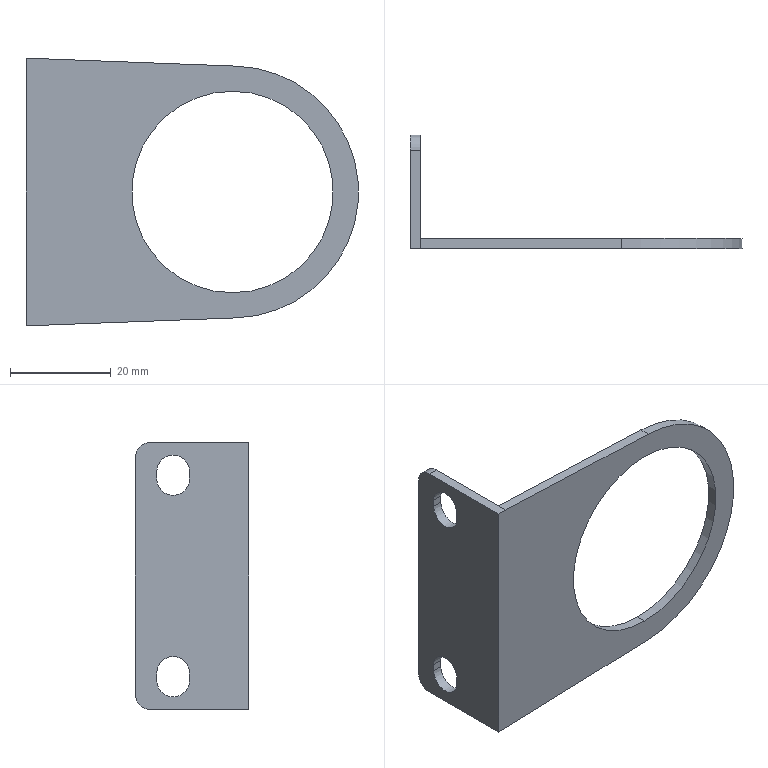Part | SolidWorks | features BaseBody 1 | 1 solid | 24 faces | box 66 x 22.5 x 53 mm | volume 5674 mm3 | plane 13 | cylinder 11 | commonest cylinder face diameters 6.5 x6 6 x2 40 x2 50 x1
STEP:
#1=CARTESIAN_POINT('',(0.,33.,20.));
#2=VERTEX_POINT('',#1);
#3=CARTESIAN_POINT('',(0.,33.,-20.));
#4=VERTEX_POINT('',#3);
#5=CARTESIAN_POINT('',(0.,33.,0.));
#6=DIRECTION('',(0.,-1.,0.));
#7=DIRECTION('',(0.,0.,-1.));
#8=AXIS2_PLACEMENT_3D('',#5,#6,#7);
#9=CIRCLE('',#8,20.);
#10=EDGE_CURVE('',#2,#4,#9,.T.);
#11=ORIENTED_EDGE('',*,*,#10,.F.);
#12=CARTESIAN_POINT('',(0.,31.,20.));
#13=VERTEX_POINT('',#12);
#14=CARTESIAN_POINT('',(0.,31.,20.));
#15=DIRECTION('',(0.,-1.,0.));
#16=VECTOR('',#15,1000.);
#17=LINE('',#14,#16);
#18=EDGE_CURVE('',#2,#13,#17,.T.);
#19=ORIENTED_EDGE('',*,*,#18,.T.);
#20=CARTESIAN_POINT('',(0.,31.,-20.));
#21=VERTEX_POINT('',#20);
#22=CARTESIAN_POINT('',(0.,31.,0.));
#23=DIRECTION('',(0.,1.,0.));
#24=DIRECTION('',(0.,0.,-1.));
#25=AXIS2_PLACEMENT_3D('',#22,#23,#24);
#26=CIRCLE('',#25,20.);
#27=EDGE_CURVE('',#21,#13,#26,.T.);
#28=ORIENTED_EDGE('',*,*,#27,.F.);
#29=CARTESIAN_POINT('',(0.,31.,-20.));
#30=DIRECTION('',(0.,-1.,0.));
#31=VECTOR('',#30,1000.);
#32=LINE('',#29,#31);
#33=EDGE_CURVE('',#4,#21,#32,.T.);
#34=ORIENTED_EDGE('',*,*,#33,.F.);
#35=EDGE_LOOP('',(#11,#19,#28,#34));
#36=FACE_OUTER_BOUND('',#35,.T.);
#37=CARTESIAN_POINT('',(0.,31.,0.));
#38=DIRECTION('',(0.,-1.,0.));
#39=DIRECTION('',(0.,0.,-1.));
#40=AXIS2_PLACEMENT_3D('',#37,#38,#39);
#41=CYLINDRICAL_SURFACE('',#40,20.);
#42=ADVANCED_FACE('',(#36),#41,.F.);
#43=CARTESIAN_POINT('',(-39.,46.,24.));
#44=VERTEX_POINT('',#43);
#45=CARTESIAN_POINT('',(-39.,49.25,20.75));
#46=VERTEX_POINT('',#45);
#47=CARTESIAN_POINT('',(-39.,46.,20.75));
#48=DIRECTION('',(-1.,0.,0.));
#49=DIRECTION('',(0.,0.,1.));
#50=AXIS2_PLACEMENT_3D('',#47,#48,#49);
#51=CIRCLE('',#50,3.25);
#52=EDGE_CURVE('',#44,#46,#51,.T.);
#53=ORIENTED_EDGE('',*,*,#52,.F.);
#54=CARTESIAN_POINT('',(-41.,46.,24.));
#55=VERTEX_POINT('',#54);
#56=CARTESIAN_POINT('',(-41.,46.,24.));
#57=DIRECTION('',(-1.,0.,0.));
#58=VECTOR('',#57,1000.);
#59=LINE('',#56,#58);
#60=EDGE_CURVE('',#44,#55,#59,.T.);
#61=ORIENTED_EDGE('',*,*,#60,.T.);
#62=CARTESIAN_POINT('',(-41.,49.25,20.75));
#63=VERTEX_POINT('',#62);
#64=CARTESIAN_POINT('',(-41.,46.,20.75));
#65=DIRECTION('',(-1.,0.,0.));
#66=DIRECTION('',(0.,0.,1.));
#67=AXIS2_PLACEMENT_3D('',#64,#65,#66);
#68=CIRCLE('',#67,3.25);
#69=EDGE_CURVE('',#55,#63,#68,.T.);
#70=ORIENTED_EDGE('',*,*,#69,.T.);
#71=CARTESIAN_POINT('',(-41.,49.25,20.75));
#72=DIRECTION('',(-1.,0.,0.));
#73=VECTOR('',#72,1000.);
#74=LINE('',#71,#73);
#75=EDGE_CURVE('',#46,#63,#74,.T.);
#76=ORIENTED_EDGE('',*,*,#75,.F.);
#77=EDGE_LOOP('',(#53,#61,#70,#76));
#78=FACE_OUTER_BOUND('',#77,.T.);
#79=CARTESIAN_POINT('',(-41.,46.,20.75));
#80=DIRECTION('',(-1.,0.,0.));
#81=DIRECTION('',(0.,0.,1.));
#82=AXIS2_PLACEMENT_3D('',#79,#80,#81);
#83=CYLINDRICAL_SURFACE('',#82,3.25);
#84=ADVANCED_FACE('',(#78),#83,.F.);
#85=CARTESIAN_POINT('',(-39.,46.,-16.));
#86=VERTEX_POINT('',#85);
#87=CARTESIAN_POINT('',(-39.,49.25,-19.25));
#88=VERTEX_POINT('',#87);
#89=CARTESIAN_POINT('',(-39.,46.,-19.25));
#90=DIRECTION('',(-1.,0.,0.));
#91=DIRECTION('',(0.,0.,1.));
#92=AXIS2_PLACEMENT_3D('',#89,#90,#91);
#93=CIRCLE('',#92,3.25);
#94=EDGE_CURVE('',#86,#88,#93,.T.);
#95=ORIENTED_EDGE('',*,*,#94,.F.);
#96=CARTESIAN_POINT('',(-41.,46.,-16.));
#97=VERTEX_POINT('',#96);
#98=CARTESIAN_POINT('',(-41.,46.,-16.));
#99=DIRECTION('',(-1.,0.,0.));
#100=VECTOR('',#99,1000.);
#101=LINE('',#98,#100);
#102=EDGE_CURVE('',#86,#97,#101,.T.);
#103=ORIENTED_EDGE('',*,*,#102,.T.);
#104=CARTESIAN_POINT('',(-41.,49.25,-19.25));
#105=VERTEX_POINT('',#104);
#106=CARTESIAN_POINT('',(-41.,46.,-19.25));
#107=DIRECTION('',(-1.,0.,0.));
#108=DIRECTION('',(0.,0.,1.));
#109=AXIS2_PLACEMENT_3D('',#106,#107,#108);
#110=CIRCLE('',#109,3.25);
#111=EDGE_CURVE('',#97,#105,#110,.T.);
#112=ORIENTED_EDGE('',*,*,#111,.T.);
#113=CARTESIAN_POINT('',(-41.,49.25,-19.25));
#114=DIRECTION('',(-1.,0.,0.));
#115=VECTOR('',#114,1000.);
#116=LINE('',#113,#115);
#117=EDGE_CURVE('',#88,#105,#116,.T.);
#118=ORIENTED_EDGE('',*,*,#117,.F.);
#119=EDGE_LOOP('',(#95,#103,#112,#118));
#120=FACE_OUTER_BOUND('',#119,.T.);
#121=CARTESIAN_POINT('',(-41.,46.,-19.25));
#122=DIRECTION('',(-1.,0.,0.));
#123=DIRECTION('',(0.,0.,1.));
#124=AXIS2_PLACEMENT_3D('',#121,#122,#123);
#125=CYLINDRICAL_SURFACE('',#124,3.25);
#126=ADVANCED_FACE('',(#120),#125,.F.);
#127=CARTESIAN_POINT('',(-41.,49.25,-20.75));
#128=VERTEX_POINT('',#127);
#129=CARTESIAN_POINT('',(-41.,49.25,-20.75));
#130=DIRECTION('',(0.,0.,-1.));
#131=VECTOR('',#130,1000.);
#132=LINE('',#129,#131);
#133=EDGE_CURVE('',#105,#128,#132,.T.);
#134=ORIENTED_EDGE('',*,*,#133,.T.);
#135=CARTESIAN_POINT('',(-39.,49.25,-20.75));
#136=VERTEX_POINT('',#135);
#137=CARTESIAN_POINT('',(-41.,49.25,-20.75));
#138=DIRECTION('',(1.,0.,0.));
#139=VECTOR('',#138,1000.);
#140=LINE('',#137,#139);
#141=EDGE_CURVE('',#128,#136,#140,.T.);
#142=ORIENTED_EDGE('',*,*,#141,.T.);
#143=CARTESIAN_POINT('',(-39.,49.25,-20.75));
#144=DIRECTION('',(0.,0.,1.));
#145=VECTOR('',#144,1000.);
#146=LINE('',#143,#145);
#147=EDGE_CURVE('',#136,#88,#146,.T.);
#148=ORIENTED_EDGE('',*,*,#147,.T.);
#149=ORIENTED_EDGE('',*,*,#117,.T.);
#150=EDGE_LOOP('',(#134,#142,#148,#149));
#151=FACE_OUTER_BOUND('',#150,.T.);
#152=CARTESIAN_POINT('',(-41.,49.25,-20.75));
#153=DIRECTION('',(0.,-1.,0.));
#154=DIRECTION('',(0.,0.,-1.));
#155=AXIS2_PLACEMENT_3D('',#152,#153,#154);
#156=PLANE('',#155);
#157=ADVANCED_FACE('',(#151),#156,.T.);
#158=CARTESIAN_POINT('',(-41.,42.75,-20.75));
#159=VERTEX_POINT('',#158);
#160=CARTESIAN_POINT('',(-41.,42.75,-19.25));
#161=VERTEX_POINT('',#160);
#162=CARTESIAN_POINT('',(-41.,42.75,-19.25));
#163=DIRECTION('',(0.,0.,1.));
#164=VECTOR('',#163,1000.);
#165=LINE('',#162,#164);
#166=EDGE_CURVE('',#159,#161,#165,.T.);
#167=ORIENTED_EDGE('',*,*,#166,.T.);
#168=CARTESIAN_POINT('',(-39.,42.75,-19.25));
#169=VERTEX_POINT('',#168);
#170=CARTESIAN_POINT('',(-41.,42.75,-19.25));
#171=DIRECTION('',(1.,0.,0.));
#172=VECTOR('',#171,1000.);
#173=LINE('',#170,#172);
#174=EDGE_CURVE('',#161,#169,#173,.T.);
#175=ORIENTED_EDGE('',*,*,#174,.T.);
#176=CARTESIAN_POINT('',(-39.,42.75,-20.75));
#177=VERTEX_POINT('',#176);
#178=CARTESIAN_POINT('',(-39.,42.75,-19.25));
#179=DIRECTION('',(0.,0.,-1.));
#180=VECTOR('',#179,1000.);
#181=LINE('',#178,#180);
#182=EDGE_CURVE('',#169,#177,#181,.T.);
#183=ORIENTED_EDGE('',*,*,#182,.T.);
#184=CARTESIAN_POINT('',(-41.,42.75,-20.75));
#185=DIRECTION('',(-1.,0.,0.));
#186=VECTOR('',#185,1000.);
#187=LINE('',#184,#186);
#188=EDGE_CURVE('',#177,#159,#187,.T.);
#189=ORIENTED_EDGE('',*,*,#188,.T.);
#190=EDGE_LOOP('',(#167,#175,#183,#189));
#191=FACE_OUTER_BOUND('',#190,.T.);
#192=CARTESIAN_POINT('',(-41.,42.75,-19.25));
#193=DIRECTION('',(0.,1.,0.));
#194=DIRECTION('',(1.,0.,0.));
#195=AXIS2_PLACEMENT_3D('',#192,#193,#194);
#196=PLANE('',#195);
#197=ADVANCED_FACE('',(#191),#196,.T.);
#198=CARTESIAN_POINT('',(-41.,49.25,19.25));
#199=VERTEX_POINT('',#198);
#200=CARTESIAN_POINT('',(-41.,49.25,19.25));
#201=DIRECTION('',(0.,0.,-1.));
#202=VECTOR('',#201,1000.);
#203=LINE('',#200,#202);
#204=EDGE_CURVE('',#63,#199,#203,.T.);
#205=ORIENTED_EDGE('',*,*,#204,.T.);
#206=CARTESIAN_POINT('',(-39.,49.25,19.25));
#207=VERTEX_POINT('',#206);
#208=CARTESIAN_POINT('',(-41.,49.25,19.25));
#209=DIRECTION('',(1.,0.,0.));
#210=VECTOR('',#209,1000.);
#211=LINE('',#208,#210);
#212=EDGE_CURVE('',#199,#207,#211,.T.);
#213=ORIENTED_EDGE('',*,*,#212,.T.);
#214=CARTESIAN_POINT('',(-39.,49.25,19.25));
#215=DIRECTION('',(0.,0.,1.));
#216=VECTOR('',#215,1000.);
#217=LINE('',#214,#216);
#218=EDGE_CURVE('',#207,#46,#217,.T.);
#219=ORIENTED_EDGE('',*,*,#218,.T.);
#220=ORIENTED_EDGE('',*,*,#75,.T.);
#221=EDGE_LOOP('',(#205,#213,#219,#220));
#222=FACE_OUTER_BOUND('',#221,.T.);
#223=CARTESIAN_POINT('',(-41.,49.25,19.25));
#224=DIRECTION('',(0.,-1.,0.));
#225=DIRECTION('',(0.,0.,-1.));
#226=AXIS2_PLACEMENT_3D('',#223,#224,#225);
#227=PLANE('',#226);
#228=ADVANCED_FACE('',(#222),#227,.T.);
#229=CARTESIAN_POINT('',(-41.,42.75,19.25));
#230=VERTEX_POINT('',#229);
#231=CARTESIAN_POINT('',(-41.,42.75,20.75));
#232=VERTEX_POINT('',#231);
#233=CARTESIAN_POINT('',(-41.,42.75,20.75));
#234=DIRECTION('',(0.,0.,1.));
#235=VECTOR('',#234,1000.);
#236=LINE('',#233,#235);
#237=EDGE_CURVE('',#230,#232,#236,.T.);
#238=ORIENTED_EDGE('',*,*,#237,.T.);
#239=CARTESIAN_POINT('',(-39.,42.75,20.75));
#240=VERTEX_POINT('',#239);
#241=CARTESIAN_POINT('',(-41.,42.75,20.75));
#242=DIRECTION('',(1.,0.,0.));
#243=VECTOR('',#242,1000.);
#244=LINE('',#241,#243);
#245=EDGE_CURVE('',#232,#240,#244,.T.);
#246=ORIENTED_EDGE('',*,*,#245,.T.);
#247=CARTESIAN_POINT('',(-39.,42.75,19.25));
#248=VERTEX_POINT('',#247);
#249=CARTESIAN_POINT('',(-39.,42.75,20.75));
#250=DIRECTION('',(0.,0.,-1.));
#251=VECTOR('',#250,1000.);
#252=LINE('',#249,#251);
#253=EDGE_CURVE('',#240,#248,#252,.T.);
#254=ORIENTED_EDGE('',*,*,#253,.T.);
#255=CARTESIAN_POINT('',(-41.,42.75,19.25));
#256=DIRECTION('',(-1.,0.,0.));
#257=VECTOR('',#256,1000.);
#258=LINE('',#255,#257);
#259=EDGE_CURVE('',#248,#230,#258,.T.);
#260=ORIENTED_EDGE('',*,*,#259,.T.);
#261=EDGE_LOOP('',(#238,#246,#254,#260));
#262=FACE_OUTER_BOUND('',#261,.T.);
#263=CARTESIAN_POINT('',(-41.,42.75,20.75));
#264=DIRECTION('',(0.,1.,0.));
#265=DIRECTION('',(1.,0.,0.));
#266=AXIS2_PLACEMENT_3D('',#263,#264,#265);
#267=PLANE('',#266);
#268=ADVANCED_FACE('',(#262),#267,.T.);
#269=CARTESIAN_POINT('',(-41.,53.5,-23.5));
#270=VERTEX_POINT('',#269);
#271=CARTESIAN_POINT('',(-41.,53.5,23.5));
#272=VERTEX_POINT('',#271);
#273=CARTESIAN_POINT('',(-41.,53.5,0.));
#274=DIRECTION('',(0.,0.,1.));
#275=VECTOR('',#274,1000.);
#276=LINE('',#273,#275);
#277=EDGE_CURVE('',#270,#272,#276,.T.);
#278=ORIENTED_EDGE('',*,*,#277,.T.);
#279=CARTESIAN_POINT('',(-39.,53.5,23.5));
#280=VERTEX_POINT('',#279);
#281=CARTESIAN_POINT('',(-41.,53.5,23.5));
#282=DIRECTION('',(-1.,0.,0.));
#283=VECTOR('',#282,1000.);
#284=LINE('',#281,#283);
#285=EDGE_CURVE('',#280,#272,#284,.T.);
#286=ORIENTED_EDGE('',*,*,#285,.F.);
#287=CARTESIAN_POINT('',(-39.,53.5,-23.5));
#288=VERTEX_POINT('',#287);
#289=CARTESIAN_POINT('',(-39.,53.5,0.));
#290=DIRECTION('',(0.,0.,1.));
#291=VECTOR('',#290,1000.);
#292=LINE('',#289,#291);
#293=EDGE_CURVE('',#288,#280,#292,.T.);
#294=ORIENTED_EDGE('',*,*,#293,.F.);
#295=CARTESIAN_POINT('',(-41.,53.5,-23.5));
#296=DIRECTION('',(1.,0.,0.));
#297=VECTOR('',#296,1000.);
#298=LINE('',#295,#297);
#299=EDGE_CURVE('',#270,#288,#298,.T.);
#300=ORIENTED_EDGE('',*,*,#299,.F.);
#301=EDGE_LOOP('',(#278,#286,#294,#300));
#302=FACE_OUTER_BOUND('',#301,.T.);
#303=CARTESIAN_POINT('',(-41.,53.5,23.5));
#304=DIRECTION('',(0.,1.,0.));
#305=DIRECTION('',(1.,0.,0.));
#306=AXIS2_PLACEMENT_3D('',#303,#304,#305);
#307=PLANE('',#306);
#308=ADVANCED_FACE('',(#302),#307,.T.);
#309=CARTESIAN_POINT('',(-41.,50.5,26.5));
#310=VERTEX_POINT('',#309);
#311=CARTESIAN_POINT('',(-41.,50.5,23.5));
#312=DIRECTION('',(1.,0.,0.));
#313=DIRECTION('',(0.,0.,1.));
#314=AXIS2_PLACEMENT_3D('',#311,#312,#313);
#315=CIRCLE('',#314,3.);
#316=EDGE_CURVE('',#272,#310,#315,.T.);
#317=ORIENTED_EDGE('',*,*,#316,.T.);
#318=CARTESIAN_POINT('',(-39.,50.5,26.5));
#319=VERTEX_POINT('',#318);
#320=CARTESIAN_POINT('',(-41.,50.5,26.5));
#321=DIRECTION('',(-1.,0.,0.));
#322=VECTOR('',#321,1000.);
#323=LINE('',#320,#322);
#324=EDGE_CURVE('',#319,#310,#323,.T.);
#325=ORIENTED_EDGE('',*,*,#324,.F.);
#326=CARTESIAN_POINT('',(-39.,50.5,23.5));
#327=DIRECTION('',(1.,0.,0.));
#328=DIRECTION('',(0.,0.,1.));
#329=AXIS2_PLACEMENT_3D('',#326,#327,#328);
#330=CIRCLE('',#329,3.);
#331=EDGE_CURVE('',#280,#319,#330,.T.);
#332=ORIENTED_EDGE('',*,*,#331,.F.);
#333=ORIENTED_EDGE('',*,*,#285,.T.);
#334=EDGE_LOOP('',(#317,#325,#332,#333));
#335=FACE_OUTER_BOUND('',#334,.T.);
#336=CARTESIAN_POINT('',(-41.,50.5,23.5));
#337=DIRECTION('',(-1.,0.,0.));
#338=DIRECTION('',(0.,0.,1.));
#339=AXIS2_PLACEMENT_3D('',#336,#337,#338);
#340=CYLINDRICAL_SURFACE('',#339,3.);
#341=ADVANCED_FACE('',(#335),#340,.T.);
#342=ORIENTED_EDGE('',*,*,#141,.F.);
#343=CARTESIAN_POINT('',(-41.,46.,-20.75));
#344=DIRECTION('',(-1.,0.,0.));
#345=DIRECTION('',(0.,0.,1.));
#346=AXIS2_PLACEMENT_3D('',#343,#344,#345);
#347=CIRCLE('',#346,3.25);
#348=EDGE_CURVE('',#128,#159,#347,.T.);
#349=ORIENTED_EDGE('',*,*,#348,.T.);
#350=ORIENTED_EDGE('',*,*,#188,.F.);
#351=CARTESIAN_POINT('',(-39.,46.,-20.75));
#352=DIRECTION('',(-1.,0.,0.));
#353=DIRECTION('',(0.,0.,1.));
#354=AXIS2_PLACEMENT_3D('',#351,#352,#353);
#355=CIRCLE('',#354,3.25);
#356=EDGE_CURVE('',#136,#177,#355,.T.);
#357=ORIENTED_EDGE('',*,*,#356,.F.);
#358=EDGE_LOOP('',(#342,#349,#350,#357));
#359=FACE_OUTER_BOUND('',#358,.T.);
#360=CARTESIAN_POINT('',(-41.,46.,-20.75));
#361=DIRECTION('',(-1.,0.,0.));
#362=DIRECTION('',(0.,0.,1.));
#363=AXIS2_PLACEMENT_3D('',#360,#361,#362);
#364=CYLINDRICAL_SURFACE('',#363,3.25);
#365=ADVANCED_FACE('',(#359),#364,.F.);
#366=ORIENTED_EDGE('',*,*,#212,.F.);
#367=CARTESIAN_POINT('',(-41.,46.,19.25));
#368=DIRECTION('',(-1.,0.,0.));
#369=DIRECTION('',(0.,0.,1.));
#370=AXIS2_PLACEMENT_3D('',#367,#368,#369);
#371=CIRCLE('',#370,3.25);
#372=EDGE_CURVE('',#199,#230,#371,.T.);
#373=ORIENTED_EDGE('',*,*,#372,.T.);
#374=ORIENTED_EDGE('',*,*,#259,.F.);
#375=CARTESIAN_POINT('',(-39.,46.,19.25));
#376=DIRECTION('',(-1.,0.,0.));
#377=DIRECTION('',(0.,0.,1.));
#378=AXIS2_PLACEMENT_3D('',#375,#376,#377);
#379=CIRCLE('',#378,3.25);
#380=EDGE_CURVE('',#207,#248,#379,.T.);
#381=ORIENTED_EDGE('',*,*,#380,.F.);
#382=EDGE_LOOP('',(#366,#373,#374,#381));
#383=FACE_OUTER_BOUND('',#382,.T.);
#384=CARTESIAN_POINT('',(-41.,46.,19.25));
#385=DIRECTION('',(-1.,0.,0.));
#386=DIRECTION('',(0.,0.,1.));
#387=AXIS2_PLACEMENT_3D('',#384,#385,#386);
#388=CYLINDRICAL_SURFACE('',#387,3.25);
#389=ADVANCED_FACE('',(#383),#388,.F.);
#390=ORIENTED_EDGE('',*,*,#380,.T.);
#391=ORIENTED_EDGE('',*,*,#253,.F.);
#392=CARTESIAN_POINT('',(-39.,46.,20.75));
#393=DIRECTION('',(-1.,0.,0.));
#394=DIRECTION('',(0.,0.,1.));
#395=AXIS2_PLACEMENT_3D('',#392,#393,#394);
#396=CIRCLE('',#395,3.25);
#397=EDGE_CURVE('',#240,#44,#396,.T.);
#398=ORIENTED_EDGE('',*,*,#397,.T.);
#399=ORIENTED_EDGE('',*,*,#52,.T.);
#400=ORIENTED_EDGE('',*,*,#218,.F.);
#401=EDGE_LOOP('',(#390,#391,#398,#399,#400));
#402=FACE_BOUND('',#401,.T.);
#403=ORIENTED_EDGE('',*,*,#356,.T.);
#404=ORIENTED_EDGE('',*,*,#182,.F.);
#405=CARTESIAN_POINT('',(-39.,46.,-19.25));
#406=DIRECTION('',(-1.,0.,0.));
#407=DIRECTION('',(0.,0.,1.));
#408=AXIS2_PLACEMENT_3D('',#405,#406,#407);
#409=CIRCLE('',#408,3.25);
#410=EDGE_CURVE('',#169,#86,#409,.T.);
#411=ORIENTED_EDGE('',*,*,#410,.T.);
#412=ORIENTED_EDGE('',*,*,#94,.T.);
#413=ORIENTED_EDGE('',*,*,#147,.F.);
#414=EDGE_LOOP('',(#403,#404,#411,#412,#413));
#415=FACE_BOUND('',#414,.T.);
#416=ORIENTED_EDGE('',*,*,#331,.T.);
#417=CARTESIAN_POINT('',(-39.,33.,26.5));
#418=VERTEX_POINT('',#417);
#419=CARTESIAN_POINT('',(-39.,31.,26.5));
#420=DIRECTION('',(0.,1.,0.));
#421=VECTOR('',#420,1000.);
#422=LINE('',#419,#421);
#423=EDGE_CURVE('',#418,#319,#422,.T.);
#424=ORIENTED_EDGE('',*,*,#423,.F.);
#425=CARTESIAN_POINT('',(-39.,33.,-26.5));
#426=VERTEX_POINT('',#425);
#427=CARTESIAN_POINT('',(-39.,33.,0.));
#428=DIRECTION('',(0.,0.,1.));
#429=VECTOR('',#428,1000.);
#430=LINE('',#427,#429);
#431=EDGE_CURVE('',#426,#418,#430,.T.);
#432=ORIENTED_EDGE('',*,*,#431,.F.);
#433=CARTESIAN_POINT('',(-39.,50.5,-26.5));
#434=VERTEX_POINT('',#433);
#435=CARTESIAN_POINT('',(-39.,50.5,-26.5));
#436=DIRECTION('',(0.,-1.,0.));
#437=VECTOR('',#436,1000.);
#438=LINE('',#435,#437);
#439=EDGE_CURVE('',#434,#426,#438,.T.);
#440=ORIENTED_EDGE('',*,*,#439,.F.);
#441=CARTESIAN_POINT('',(-39.,50.5,-23.5));
#442=DIRECTION('',(-1.,0.,0.));
#443=DIRECTION('',(0.,0.,1.));
#444=AXIS2_PLACEMENT_3D('',#441,#442,#443);
#445=CIRCLE('',#444,3.);
#446=EDGE_CURVE('',#288,#434,#445,.T.);
#447=ORIENTED_EDGE('',*,*,#446,.F.);
#448=ORIENTED_EDGE('',*,*,#293,.T.);
#449=EDGE_LOOP('',(#416,#424,#432,#440,#447,#448));
#450=FACE_OUTER_BOUND('',#449,.T.);
#451=CARTESIAN_POINT('',(-39.,31.,0.));
#452=DIRECTION('',(1.,0.,0.));
#453=DIRECTION('',(0.,1.,0.));
#454=AXIS2_PLACEMENT_3D('',#451,#452,#453);
#455=PLANE('',#454);
#456=ADVANCED_FACE('',(#402,#415,#450),#455,.T.);
#457=CARTESIAN_POINT('',(-41.,50.5,-26.5));
#458=VERTEX_POINT('',#457);
#459=CARTESIAN_POINT('',(-41.,50.5,-23.5));
#460=DIRECTION('',(1.,0.,0.));
#461=DIRECTION('',(0.,0.,1.));
#462=AXIS2_PLACEMENT_3D('',#459,#460,#461);
#463=CIRCLE('',#462,3.);
#464=EDGE_CURVE('',#458,#270,#463,.T.);
#465=ORIENTED_EDGE('',*,*,#464,.T.);
#466=ORIENTED_EDGE('',*,*,#299,.T.);
#467=ORIENTED_EDGE('',*,*,#446,.T.);
#468=CARTESIAN_POINT('',(-41.,50.5,-26.5));
#469=DIRECTION('',(1.,0.,0.));
#470=VECTOR('',#469,1000.);
#471=LINE('',#468,#470);
#472=EDGE_CURVE('',#458,#434,#471,.T.);
#473=ORIENTED_EDGE('',*,*,#472,.F.);
#474=EDGE_LOOP('',(#465,#466,#467,#473));
#475=FACE_OUTER_BOUND('',#474,.T.);
#476=CARTESIAN_POINT('',(-41.,50.5,-23.5));
#477=DIRECTION('',(-1.,0.,0.));
#478=DIRECTION('',(0.,0.,1.));
#479=AXIS2_PLACEMENT_3D('',#476,#477,#478);
#480=CYLINDRICAL_SURFACE('',#479,3.);
#481=ADVANCED_FACE('',(#475),#480,.T.);
#482=CARTESIAN_POINT('',(0.,33.,0.));
#483=DIRECTION('',(0.,-1.,0.));
#484=DIRECTION('',(0.,0.,-1.));
#485=AXIS2_PLACEMENT_3D('',#482,#483,#484);
#486=CIRCLE('',#485,20.);
#487=EDGE_CURVE('',#4,#2,#486,.T.);
#488=ORIENTED_EDGE('',*,*,#487,.T.);
#489=ORIENTED_EDGE('',*,*,#10,.T.);
#490=EDGE_LOOP('',(#488,#489));
#491=FACE_BOUND('',#490,.T.);
#492=CARTESIAN_POINT('',(0.9493,33.,-24.982));
#493=VERTEX_POINT('',#492);
#494=CARTESIAN_POINT('',(0.9493,33.,24.982));
#495=VERTEX_POINT('',#494);
#496=CARTESIAN_POINT('',(0.,33.,0.));
#497=DIRECTION('',(0.,-1.,0.));
#498=DIRECTION('',(0.,0.,-1.));
#499=AXIS2_PLACEMENT_3D('',#496,#497,#498);
#500=CIRCLE('',#499,25.);
#501=EDGE_CURVE('',#493,#495,#500,.T.);
#502=ORIENTED_EDGE('',*,*,#501,.F.);
#503=CARTESIAN_POINT('',(-39.,33.,-26.5));
#504=DIRECTION('',(0.9993,0.,0.03797));
#505=VECTOR('',#504,1000.);
#506=LINE('',#503,#505);
#507=EDGE_CURVE('',#426,#493,#506,.T.);
#508=ORIENTED_EDGE('',*,*,#507,.F.);
#509=ORIENTED_EDGE('',*,*,#431,.T.);
#510=CARTESIAN_POINT('',(0.9493,33.,24.982));
#511=DIRECTION('',(-0.9993,0.,0.03797));
#512=VECTOR('',#511,1000.);
#513=LINE('',#510,#512);
#514=EDGE_CURVE('',#495,#418,#513,.T.);
#515=ORIENTED_EDGE('',*,*,#514,.F.);
#516=EDGE_LOOP('',(#502,#508,#509,#515));
#517=FACE_OUTER_BOUND('',#516,.T.);
#518=CARTESIAN_POINT('',(0.,33.,0.));
#519=DIRECTION('',(0.,1.,0.));
#520=DIRECTION('',(1.,0.,0.));
#521=AXIS2_PLACEMENT_3D('',#518,#519,#520);
#522=PLANE('',#521);
#523=ADVANCED_FACE('',(#491,#517),#522,.T.);
#524=CARTESIAN_POINT('',(-41.,31.,26.5));
#525=VERTEX_POINT('',#524);
#526=CARTESIAN_POINT('',(-41.,31.,26.5));
#527=DIRECTION('',(0.,-1.,0.));
#528=VECTOR('',#527,1000.);
#529=LINE('',#526,#528);
#530=EDGE_CURVE('',#310,#525,#529,.T.);
#531=ORIENTED_EDGE('',*,*,#530,.T.);
#532=CARTESIAN_POINT('',(-39.,31.,26.5));
#533=VERTEX_POINT('',#532);
#534=CARTESIAN_POINT('',(-41.,31.,26.5));
#535=DIRECTION('',(-1.,0.,0.));
#536=VECTOR('',#535,1000.);
#537=LINE('',#534,#536);
#538=EDGE_CURVE('',#533,#525,#537,.T.);
#539=ORIENTED_EDGE('',*,*,#538,.F.);
#540=CARTESIAN_POINT('',(-39.,31.,26.5));
#541=DIRECTION('',(0.,-1.,0.));
#542=VECTOR('',#541,1000.);
#543=LINE('',#540,#542);
#544=EDGE_CURVE('',#418,#533,#543,.T.);
#545=ORIENTED_EDGE('',*,*,#544,.F.);
#546=ORIENTED_EDGE('',*,*,#423,.T.);
#547=ORIENTED_EDGE('',*,*,#324,.T.);
#548=EDGE_LOOP('',(#531,#539,#545,#546,#547));
#549=FACE_OUTER_BOUND('',#548,.T.);
#550=CARTESIAN_POINT('',(-41.,31.,26.5));
#551=DIRECTION('',(0.,0.,1.));
#552=DIRECTION('',(1.,0.,0.));
#553=AXIS2_PLACEMENT_3D('',#550,#551,#552);
#554=PLANE('',#553);
#555=ADVANCED_FACE('',(#549),#554,.T.);
#556=CARTESIAN_POINT('',(-41.,46.,-19.25));
#557=DIRECTION('',(-1.,0.,0.));
#558=DIRECTION('',(0.,0.,1.));
#559=AXIS2_PLACEMENT_3D('',#556,#557,#558);
#560=CIRCLE('',#559,3.25);
#561=EDGE_CURVE('',#161,#97,#560,.T.);
#562=ORIENTED_EDGE('',*,*,#561,.F.);
#563=ORIENTED_EDGE('',*,*,#166,.F.);
#564=ORIENTED_EDGE('',*,*,#348,.F.);
#565=ORIENTED_EDGE('',*,*,#133,.F.);
#566=ORIENTED_EDGE('',*,*,#111,.F.);
#567=EDGE_LOOP('',(#562,#563,#564,#565,#566));
#568=FACE_BOUND('',#567,.T.);
#569=CARTESIAN_POINT('',(-41.,46.,20.75));
#570=DIRECTION('',(-1.,0.,0.));
#571=DIRECTION('',(0.,0.,1.));
#572=AXIS2_PLACEMENT_3D('',#569,#570,#571);
#573=CIRCLE('',#572,3.25);
#574=EDGE_CURVE('',#232,#55,#573,.T.);
#575=ORIENTED_EDGE('',*,*,#574,.F.);
#576=ORIENTED_EDGE('',*,*,#237,.F.);
#577=ORIENTED_EDGE('',*,*,#372,.F.);
#578=ORIENTED_EDGE('',*,*,#204,.F.);
#579=ORIENTED_EDGE('',*,*,#69,.F.);
#580=EDGE_LOOP('',(#575,#576,#577,#578,#579));
#581=FACE_BOUND('',#580,.T.);
#582=ORIENTED_EDGE('',*,*,#530,.F.);
#583=ORIENTED_EDGE('',*,*,#316,.F.);
#584=ORIENTED_EDGE('',*,*,#277,.F.);
#585=ORIENTED_EDGE('',*,*,#464,.F.);
#586=CARTESIAN_POINT('',(-41.,31.,-26.5));
#587=VERTEX_POINT('',#586);
#588=CARTESIAN_POINT('',(-41.,50.5,-26.5));
#589=DIRECTION('',(0.,1.,0.));
#590=VECTOR('',#589,1000.);
#591=LINE('',#588,#590);
#592=EDGE_CURVE('',#587,#458,#591,.T.);
#593=ORIENTED_EDGE('',*,*,#592,.F.);
#594=CARTESIAN_POINT('',(-41.,31.,-26.5));
#595=DIRECTION('',(0.,0.,-1.));
#596=VECTOR('',#595,1000.);
#597=LINE('',#594,#596);
#598=EDGE_CURVE('',#525,#587,#597,.T.);
#599=ORIENTED_EDGE('',*,*,#598,.F.);
#600=EDGE_LOOP('',(#582,#583,#584,#585,#593,#599));
#601=FACE_OUTER_BOUND('',#600,.T.);
#602=CARTESIAN_POINT('',(-41.,31.,0.));
#603=DIRECTION('',(1.,0.,0.));
#604=DIRECTION('',(0.,1.,0.));
#605=AXIS2_PLACEMENT_3D('',#602,#603,#604);
#606=PLANE('',#605);
#607=ADVANCED_FACE('',(#568,#581,#601),#606,.F.);
#608=ORIENTED_EDGE('',*,*,#592,.T.);
#609=ORIENTED_EDGE('',*,*,#472,.T.);
#610=ORIENTED_EDGE('',*,*,#439,.T.);
#611=CARTESIAN_POINT('',(-39.,31.,-26.5));
#612=VERTEX_POINT('',#611);
#613=CARTESIAN_POINT('',(-39.,31.,-26.5));
#614=DIRECTION('',(0.,1.,0.));
#615=VECTOR('',#614,1000.);
#616=LINE('',#613,#615);
#617=EDGE_CURVE('',#612,#426,#616,.T.);
#618=ORIENTED_EDGE('',*,*,#617,.F.);
#619=CARTESIAN_POINT('',(-41.,31.,-26.5));
#620=DIRECTION('',(1.,0.,0.));
#621=VECTOR('',#620,1000.);
#622=LINE('',#619,#621);
#623=EDGE_CURVE('',#587,#612,#622,.T.);
#624=ORIENTED_EDGE('',*,*,#623,.F.);
#625=EDGE_LOOP('',(#608,#609,#610,#618,#624));
#626=FACE_OUTER_BOUND('',#625,.T.);
#627=CARTESIAN_POINT('',(-41.,50.5,-26.5));
#628=DIRECTION('',(0.,0.,-1.));
#629=DIRECTION('',(0.,-1.,0.));
#630=AXIS2_PLACEMENT_3D('',#627,#628,#629);
#631=PLANE('',#630);
#632=ADVANCED_FACE('',(#626),#631,.T.);
#633=CARTESIAN_POINT('',(0.9493,31.,-24.982));
#634=VERTEX_POINT('',#633);
#635=CARTESIAN_POINT('',(-39.,31.,-26.5));
#636=DIRECTION('',(0.9993,0.,0.03797));
#637=VECTOR('',#636,1000.);
#638=LINE('',#635,#637);
#639=EDGE_CURVE('',#612,#634,#638,.T.);
#640=ORIENTED_EDGE('',*,*,#639,.F.);
#641=ORIENTED_EDGE('',*,*,#617,.T.);
#642=ORIENTED_EDGE('',*,*,#507,.T.);
#643=CARTESIAN_POINT('',(0.9493,31.,-24.982));
#644=DIRECTION('',(0.,1.,0.));
#645=VECTOR('',#644,1000.);
#646=LINE('',#643,#645);
#647=EDGE_CURVE('',#634,#493,#646,.T.);
#648=ORIENTED_EDGE('',*,*,#647,.F.);
#649=EDGE_LOOP('',(#640,#641,#642,#648));
#650=FACE_OUTER_BOUND('',#649,.T.);
#651=CARTESIAN_POINT('',(-39.,31.,-26.5));
#652=DIRECTION('',(0.03797,0.,-0.9993));
#653=DIRECTION('',(0.,-1.,0.));
#654=AXIS2_PLACEMENT_3D('',#651,#652,#653);
#655=PLANE('',#654);
#656=ADVANCED_FACE('',(#650),#655,.T.);
#657=CARTESIAN_POINT('',(0.9493,31.,24.982));
#658=VERTEX_POINT('',#657);
#659=CARTESIAN_POINT('',(0.,31.,0.));
#660=DIRECTION('',(0.,-1.,0.));
#661=DIRECTION('',(0.,0.,-1.));
#662=AXIS2_PLACEMENT_3D('',#659,#660,#661);
#663=CIRCLE('',#662,25.);
#664=EDGE_CURVE('',#634,#658,#663,.T.);
#665=ORIENTED_EDGE('',*,*,#664,.F.);
#666=ORIENTED_EDGE('',*,*,#647,.T.);
#667=ORIENTED_EDGE('',*,*,#501,.T.);
#668=CARTESIAN_POINT('',(0.9493,31.,24.982));
#669=DIRECTION('',(0.,1.,0.));
#670=VECTOR('',#669,1000.);
#671=LINE('',#668,#670);
#672=EDGE_CURVE('',#658,#495,#671,.T.);
#673=ORIENTED_EDGE('',*,*,#672,.F.);
#674=EDGE_LOOP('',(#665,#666,#667,#673));
#675=FACE_OUTER_BOUND('',#674,.T.);
#676=CARTESIAN_POINT('',(0.,31.,0.));
#677=DIRECTION('',(0.,-1.,0.));
#678=DIRECTION('',(0.,0.,-1.));
#679=AXIS2_PLACEMENT_3D('',#676,#677,#678);
#680=CYLINDRICAL_SURFACE('',#679,25.);
#681=ADVANCED_FACE('',(#675),#680,.T.);
#682=CARTESIAN_POINT('',(0.9493,31.,24.982));
#683=DIRECTION('',(-0.9993,0.,0.03797));
#684=VECTOR('',#683,1000.);
#685=LINE('',#682,#684);
#686=EDGE_CURVE('',#658,#533,#685,.T.);
#687=ORIENTED_EDGE('',*,*,#686,.F.);
#688=ORIENTED_EDGE('',*,*,#672,.T.);
#689=ORIENTED_EDGE('',*,*,#514,.T.);
#690=ORIENTED_EDGE('',*,*,#544,.T.);
#691=EDGE_LOOP('',(#687,#688,#689,#690));
#692=FACE_OUTER_BOUND('',#691,.T.);
#693=CARTESIAN_POINT('',(0.9493,31.,24.982));
#694=DIRECTION('',(0.03797,0.,0.9993));
#695=DIRECTION('',(0.,-1.,0.));
#696=AXIS2_PLACEMENT_3D('',#693,#694,#695);
#697=PLANE('',#696);
#698=ADVANCED_FACE('',(#692),#697,.T.);
#699=ORIENTED_EDGE('',*,*,#27,.T.);
#700=CARTESIAN_POINT('',(0.,31.,0.));
#701=DIRECTION('',(0.,1.,0.));
#702=DIRECTION('',(0.,0.,-1.));
#703=AXIS2_PLACEMENT_3D('',#700,#701,#702);
#704=CIRCLE('',#703,20.);
#705=EDGE_CURVE('',#13,#21,#704,.T.);
#706=ORIENTED_EDGE('',*,*,#705,.T.);
#707=EDGE_LOOP('',(#699,#706));
#708=FACE_BOUND('',#707,.T.);
#709=ORIENTED_EDGE('',*,*,#664,.T.);
#710=ORIENTED_EDGE('',*,*,#686,.T.);
#711=ORIENTED_EDGE('',*,*,#538,.T.);
#712=ORIENTED_EDGE('',*,*,#598,.T.);
#713=ORIENTED_EDGE('',*,*,#623,.T.);
#714=ORIENTED_EDGE('',*,*,#639,.T.);
#715=EDGE_LOOP('',(#709,#710,#711,#712,#713,#714));
#716=FACE_OUTER_BOUND('',#715,.T.);
#717=CARTESIAN_POINT('',(-41.,31.,-26.5));
#718=DIRECTION('',(0.,-1.,0.));
#719=DIRECTION('',(0.,0.,-1.));
#720=AXIS2_PLACEMENT_3D('',#717,#718,#719);
#721=PLANE('',#720);
#722=ADVANCED_FACE('',(#708,#716),#721,.T.);
#723=ORIENTED_EDGE('',*,*,#102,.F.);
#724=ORIENTED_EDGE('',*,*,#410,.F.);
#725=ORIENTED_EDGE('',*,*,#174,.F.);
#726=ORIENTED_EDGE('',*,*,#561,.T.);
#727=EDGE_LOOP('',(#723,#724,#725,#726));
#728=FACE_OUTER_BOUND('',#727,.T.);
#729=CARTESIAN_POINT('',(-41.,46.,-19.25));
#730=DIRECTION('',(-1.,0.,0.));
#731=DIRECTION('',(0.,0.,1.));
#732=AXIS2_PLACEMENT_3D('',#729,#730,#731);
#733=CYLINDRICAL_SURFACE('',#732,3.25);
#734=ADVANCED_FACE('',(#728),#733,.F.);
#735=ORIENTED_EDGE('',*,*,#60,.F.);
#736=ORIENTED_EDGE('',*,*,#397,.F.);
#737=ORIENTED_EDGE('',*,*,#245,.F.);
#738=ORIENTED_EDGE('',*,*,#574,.T.);
#739=EDGE_LOOP('',(#735,#736,#737,#738));
#740=FACE_OUTER_BOUND('',#739,.T.);
#741=CARTESIAN_POINT('',(-41.,46.,20.75));
#742=DIRECTION('',(-1.,0.,0.));
#743=DIRECTION('',(0.,0.,1.));
#744=AXIS2_PLACEMENT_3D('',#741,#742,#743);
#745=CYLINDRICAL_SURFACE('',#744,3.25);
#746=ADVANCED_FACE('',(#740),#745,.F.);
#747=ORIENTED_EDGE('',*,*,#18,.F.);
#748=ORIENTED_EDGE('',*,*,#487,.F.);
#749=ORIENTED_EDGE('',*,*,#33,.T.);
#750=ORIENTED_EDGE('',*,*,#705,.F.);
#751=EDGE_LOOP('',(#747,#748,#749,#750));
#752=FACE_OUTER_BOUND('',#751,.T.);
#753=CARTESIAN_POINT('',(0.,31.,0.));
#754=DIRECTION('',(0.,-1.,0.));
#755=DIRECTION('',(0.,0.,-1.));
#756=AXIS2_PLACEMENT_3D('',#753,#754,#755);
#757=CYLINDRICAL_SURFACE('',#756,20.);
#758=ADVANCED_FACE('',(#752),#757,.F.);
#759=CLOSED_SHELL('',(#42,#84,#126,#157,#197,#228,#268,#308,#341,#365,#389,#456,#481,#523,#555,#607,#632,#656,#681,#698,#722,#734,#746,#758));
#760=MANIFOLD_SOLID_BREP('',#759);
#761=CARTESIAN_POINT('',(0.,0.,0.));
#762=DIRECTION('',(0.,0.,1.));
#763=DIRECTION('',(1.,0.,0.));
#764=AXIS2_PLACEMENT_3D('',#761,#762,#763);
#765=(LENGTH_UNIT()NAMED_UNIT(*)SI_UNIT(.MILLI.,.METRE.));
#766=UNCERTAINTY_MEASURE_WITH_UNIT(LENGTH_MEASURE(0.00001),#765,'','');
#767=(NAMED_UNIT(*)PLANE_ANGLE_UNIT()SI_UNIT($,.RADIAN.));
#768=(NAMED_UNIT(*)SI_UNIT($,.STERADIAN.)SOLID_ANGLE_UNIT());
#769=(GEOMETRIC_REPRESENTATION_CONTEXT(3)GLOBAL_UNCERTAINTY_ASSIGNED_CONTEXT((#766))GLOBAL_UNIT_ASSIGNED_CONTEXT((#765,#767,#768))REPRESENTATION_CONTEXT('',''));
#770=ADVANCED_BREP_SHAPE_REPRESENTATION('',(#760,#764),#769);